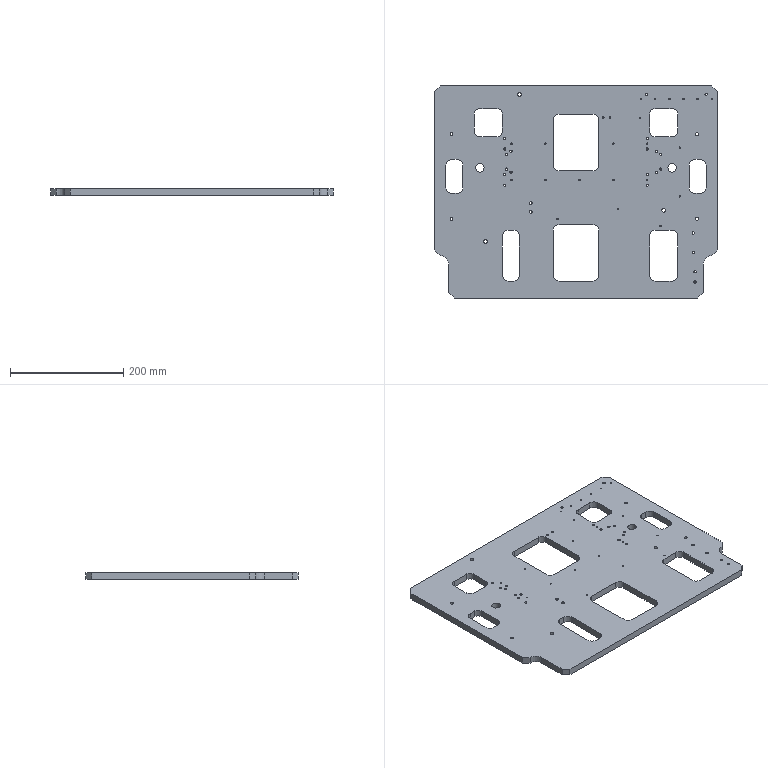Part | NX | features BREP 1 | 1 solid | 238 faces | box 500 x 375 x 12 mm | volume 1817932 mm3 | cylinder 146 | cone 46 | plane 46 | commonest cylinder face diameters 2.5 x42 20 x32 4 x28 4.2 x16 5 x12 6.5 x6